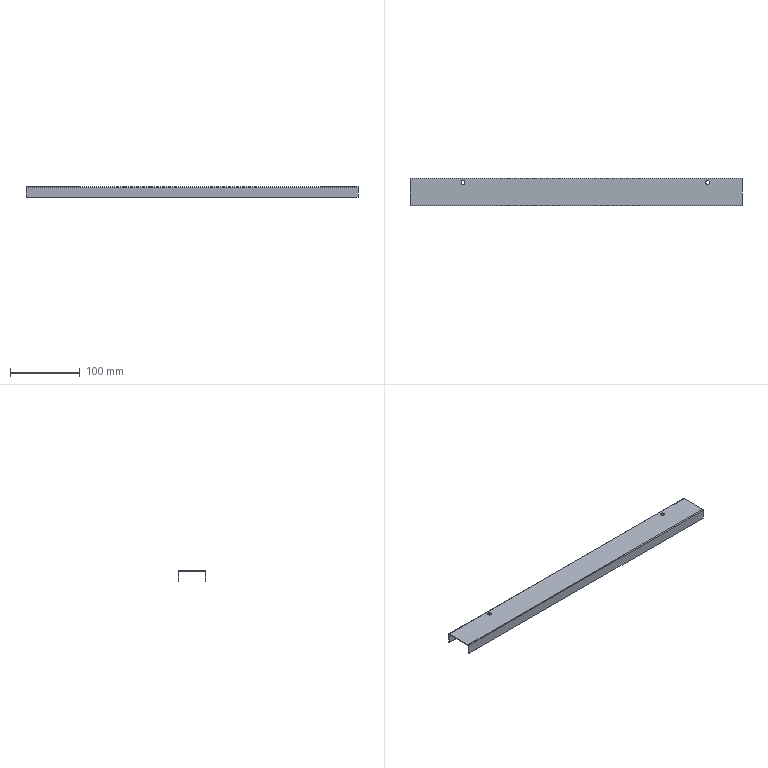Part | SolidWorks | features SplitBody 1 | 1 solid | 26 faces | box 475 x 40 x 15 mm | volume 32008 mm3 | plane 18 | cylinder 8 | commonest cylinder face diameters 5.5 x4 0.2 x2 2.2 x2
STEP:
#1=CARTESIAN_POINT('',(103.5,1393.5,274.));
#2=VERTEX_POINT('',#1);
#3=CARTESIAN_POINT('',(98.,1393.5,274.));
#4=VERTEX_POINT('',#3);
#5=CARTESIAN_POINT('',(100.75,1393.5,274.));
#6=DIRECTION('',(0.,0.,-1.));
#7=DIRECTION('',(-1.,0.,0.));
#8=AXIS2_PLACEMENT_3D('',#5,#6,#7);
#9=CIRCLE('',#8,2.75);
#10=EDGE_CURVE('',#2,#4,#9,.T.);
#11=ORIENTED_EDGE('',*,*,#10,.T.);
#12=CARTESIAN_POINT('',(98.,1393.5,275.));
#13=VERTEX_POINT('',#12);
#14=CARTESIAN_POINT('',(98.,1393.5,265.));
#15=DIRECTION('',(0.,0.,1.));
#16=VECTOR('',#15,1000.);
#17=LINE('',#14,#16);
#18=EDGE_CURVE('',#4,#13,#17,.T.);
#19=ORIENTED_EDGE('',*,*,#18,.T.);
#20=CARTESIAN_POINT('',(103.5,1393.5,275.));
#21=VERTEX_POINT('',#20);
#22=CARTESIAN_POINT('',(100.75,1393.5,275.));
#23=DIRECTION('',(0.,0.,1.));
#24=DIRECTION('',(1.,0.,0.));
#25=AXIS2_PLACEMENT_3D('',#22,#23,#24);
#26=CIRCLE('',#25,2.75);
#27=EDGE_CURVE('',#13,#21,#26,.T.);
#28=ORIENTED_EDGE('',*,*,#27,.T.);
#29=CARTESIAN_POINT('',(103.5,1393.5,265.));
#30=DIRECTION('',(0.,0.,1.));
#31=VECTOR('',#30,1000.);
#32=LINE('',#29,#31);
#33=EDGE_CURVE('',#2,#21,#32,.T.);
#34=ORIENTED_EDGE('',*,*,#33,.F.);
#35=EDGE_LOOP('',(#11,#19,#28,#34));
#36=FACE_OUTER_BOUND('',#35,.T.);
#37=CARTESIAN_POINT('',(100.75,1393.5,265.));
#38=DIRECTION('',(0.,0.,1.));
#39=DIRECTION('',(1.,0.,0.));
#40=AXIS2_PLACEMENT_3D('',#37,#38,#39);
#41=CYLINDRICAL_SURFACE('',#40,2.75);
#42=ADVANCED_FACE('',(#36),#41,.F.);
#43=CARTESIAN_POINT('',(453.5,1393.5,274.));
#44=VERTEX_POINT('',#43);
#45=CARTESIAN_POINT('',(448.,1393.5,274.));
#46=VERTEX_POINT('',#45);
#47=CARTESIAN_POINT('',(450.75,1393.5,274.));
#48=DIRECTION('',(0.,0.,-1.));
#49=DIRECTION('',(-1.,0.,0.));
#50=AXIS2_PLACEMENT_3D('',#47,#48,#49);
#51=CIRCLE('',#50,2.75);
#52=EDGE_CURVE('',#44,#46,#51,.T.);
#53=ORIENTED_EDGE('',*,*,#52,.T.);
#54=CARTESIAN_POINT('',(448.,1393.5,275.));
#55=VERTEX_POINT('',#54);
#56=CARTESIAN_POINT('',(448.,1393.5,265.));
#57=DIRECTION('',(0.,0.,1.));
#58=VECTOR('',#57,1000.);
#59=LINE('',#56,#58);
#60=EDGE_CURVE('',#46,#55,#59,.T.);
#61=ORIENTED_EDGE('',*,*,#60,.T.);
#62=CARTESIAN_POINT('',(453.5,1393.5,275.));
#63=VERTEX_POINT('',#62);
#64=CARTESIAN_POINT('',(450.75,1393.5,275.));
#65=DIRECTION('',(0.,0.,1.));
#66=DIRECTION('',(1.,0.,0.));
#67=AXIS2_PLACEMENT_3D('',#64,#65,#66);
#68=CIRCLE('',#67,2.75);
#69=EDGE_CURVE('',#55,#63,#68,.T.);
#70=ORIENTED_EDGE('',*,*,#69,.T.);
#71=CARTESIAN_POINT('',(453.5,1393.5,265.));
#72=DIRECTION('',(0.,0.,1.));
#73=VECTOR('',#72,1000.);
#74=LINE('',#71,#73);
#75=EDGE_CURVE('',#44,#63,#74,.T.);
#76=ORIENTED_EDGE('',*,*,#75,.F.);
#77=EDGE_LOOP('',(#53,#61,#70,#76));
#78=FACE_OUTER_BOUND('',#77,.T.);
#79=CARTESIAN_POINT('',(450.75,1393.5,265.));
#80=DIRECTION('',(0.,0.,1.));
#81=DIRECTION('',(1.,0.,0.));
#82=AXIS2_PLACEMENT_3D('',#79,#80,#81);
#83=CYLINDRICAL_SURFACE('',#82,2.75);
#84=ADVANCED_FACE('',(#78),#83,.F.);
#85=CARTESIAN_POINT('',(25.,1398.9,275.));
#86=VERTEX_POINT('',#85);
#87=CARTESIAN_POINT('',(25.,1398.9,274.));
#88=VERTEX_POINT('',#87);
#89=CARTESIAN_POINT('',(25.,1398.9,275.));
#90=DIRECTION('',(0.,0.,-1.));
#91=VECTOR('',#90,1000.);
#92=LINE('',#89,#91);
#93=EDGE_CURVE('',#86,#88,#92,.T.);
#94=ORIENTED_EDGE('',*,*,#93,.F.);
#95=CARTESIAN_POINT('',(25.,1400.,273.9));
#96=VERTEX_POINT('',#95);
#97=CARTESIAN_POINT('',(25.,1398.9,273.9));
#98=DIRECTION('',(1.,0.,0.));
#99=DIRECTION('',(0.,0.,1.));
#100=AXIS2_PLACEMENT_3D('',#97,#98,#99);
#101=CIRCLE('',#100,1.1);
#102=EDGE_CURVE('',#96,#86,#101,.T.);
#103=ORIENTED_EDGE('',*,*,#102,.F.);
#104=CARTESIAN_POINT('',(25.,1399.,273.9));
#105=VERTEX_POINT('',#104);
#106=CARTESIAN_POINT('',(25.,1399.,273.9));
#107=DIRECTION('',(0.,1.,0.));
#108=VECTOR('',#107,1000.);
#109=LINE('',#106,#108);
#110=EDGE_CURVE('',#105,#96,#109,.T.);
#111=ORIENTED_EDGE('',*,*,#110,.F.);
#112=CARTESIAN_POINT('',(25.,1398.9,273.9));
#113=DIRECTION('',(1.,0.,0.));
#114=DIRECTION('',(0.,0.,-1.));
#115=AXIS2_PLACEMENT_3D('',#112,#113,#114);
#116=CIRCLE('',#115,0.1);
#117=EDGE_CURVE('',#105,#88,#116,.T.);
#118=ORIENTED_EDGE('',*,*,#117,.T.);
#119=EDGE_LOOP('',(#94,#103,#111,#118));
#120=FACE_OUTER_BOUND('',#119,.T.);
#121=CARTESIAN_POINT('',(25.,1398.9,275.));
#122=DIRECTION('',(-1.,0.,0.));
#123=DIRECTION('',(0.,0.,1.));
#124=AXIS2_PLACEMENT_3D('',#121,#122,#123);
#125=PLANE('',#124);
#126=ADVANCED_FACE('',(#120),#125,.T.);
#127=CARTESIAN_POINT('',(25.,1361.1,275.));
#128=VERTEX_POINT('',#127);
#129=CARTESIAN_POINT('',(25.,1400.,275.));
#130=DIRECTION('',(0.,-1.,0.));
#131=VECTOR('',#130,1000.);
#132=LINE('',#129,#131);
#133=EDGE_CURVE('',#86,#128,#132,.T.);
#134=ORIENTED_EDGE('',*,*,#133,.F.);
#135=ORIENTED_EDGE('',*,*,#93,.T.);
#136=CARTESIAN_POINT('',(25.,1361.1,274.));
#137=VERTEX_POINT('',#136);
#138=CARTESIAN_POINT('',(25.,1400.,274.));
#139=DIRECTION('',(0.,-1.,0.));
#140=VECTOR('',#139,1000.);
#141=LINE('',#138,#140);
#142=EDGE_CURVE('',#88,#137,#141,.T.);
#143=ORIENTED_EDGE('',*,*,#142,.T.);
#144=CARTESIAN_POINT('',(25.,1361.1,274.));
#145=DIRECTION('',(0.,0.,1.));
#146=VECTOR('',#145,1000.);
#147=LINE('',#144,#146);
#148=EDGE_CURVE('',#137,#128,#147,.T.);
#149=ORIENTED_EDGE('',*,*,#148,.T.);
#150=EDGE_LOOP('',(#134,#135,#143,#149));
#151=FACE_OUTER_BOUND('',#150,.T.);
#152=CARTESIAN_POINT('',(25.,1399.,273.9));
#153=DIRECTION('',(-1.,0.,0.));
#154=DIRECTION('',(0.,0.,1.));
#155=AXIS2_PLACEMENT_3D('',#152,#153,#154);
#156=PLANE('',#155);
#157=ADVANCED_FACE('',(#151),#156,.T.);
#158=CARTESIAN_POINT('',(25.,1360.,273.9));
#159=VERTEX_POINT('',#158);
#160=CARTESIAN_POINT('',(25.,1361.,273.9));
#161=VERTEX_POINT('',#160);
#162=CARTESIAN_POINT('',(25.,1360.,273.9));
#163=DIRECTION('',(0.,1.,0.));
#164=VECTOR('',#163,1000.);
#165=LINE('',#162,#164);
#166=EDGE_CURVE('',#159,#161,#165,.T.);
#167=ORIENTED_EDGE('',*,*,#166,.F.);
#168=CARTESIAN_POINT('',(25.,1361.1,273.9));
#169=DIRECTION('',(1.,0.,0.));
#170=DIRECTION('',(0.,0.,1.));
#171=AXIS2_PLACEMENT_3D('',#168,#169,#170);
#172=CIRCLE('',#171,1.1);
#173=EDGE_CURVE('',#128,#159,#172,.T.);
#174=ORIENTED_EDGE('',*,*,#173,.F.);
#175=ORIENTED_EDGE('',*,*,#148,.F.);
#176=CARTESIAN_POINT('',(25.,1361.1,273.9));
#177=DIRECTION('',(1.,0.,0.));
#178=DIRECTION('',(0.,0.,-1.));
#179=AXIS2_PLACEMENT_3D('',#176,#177,#178);
#180=CIRCLE('',#179,0.1);
#181=EDGE_CURVE('',#137,#161,#180,.T.);
#182=ORIENTED_EDGE('',*,*,#181,.T.);
#183=EDGE_LOOP('',(#167,#174,#175,#182));
#184=FACE_OUTER_BOUND('',#183,.T.);
#185=CARTESIAN_POINT('',(25.,1360.,273.9));
#186=DIRECTION('',(-1.,0.,0.));
#187=DIRECTION('',(0.,0.,1.));
#188=AXIS2_PLACEMENT_3D('',#185,#186,#187);
#189=PLANE('',#188);
#190=ADVANCED_FACE('',(#184),#189,.T.);
#191=CARTESIAN_POINT('',(25.,1360.,260.));
#192=VERTEX_POINT('',#191);
#193=CARTESIAN_POINT('',(25.,1360.,275.));
#194=DIRECTION('',(0.,0.,-1.));
#195=VECTOR('',#194,1000.);
#196=LINE('',#193,#195);
#197=EDGE_CURVE('',#159,#192,#196,.T.);
#198=ORIENTED_EDGE('',*,*,#197,.F.);
#199=ORIENTED_EDGE('',*,*,#166,.T.);
#200=CARTESIAN_POINT('',(25.,1361.,260.));
#201=VERTEX_POINT('',#200);
#202=CARTESIAN_POINT('',(25.,1361.,275.));
#203=DIRECTION('',(0.,0.,-1.));
#204=VECTOR('',#203,1000.);
#205=LINE('',#202,#204);
#206=EDGE_CURVE('',#161,#201,#205,.T.);
#207=ORIENTED_EDGE('',*,*,#206,.T.);
#208=CARTESIAN_POINT('',(25.,1361.,260.));
#209=DIRECTION('',(0.,-1.,0.));
#210=VECTOR('',#209,1000.);
#211=LINE('',#208,#210);
#212=EDGE_CURVE('',#201,#192,#211,.T.);
#213=ORIENTED_EDGE('',*,*,#212,.T.);
#214=EDGE_LOOP('',(#198,#199,#207,#213));
#215=FACE_OUTER_BOUND('',#214,.T.);
#216=CARTESIAN_POINT('',(25.,1361.1,274.));
#217=DIRECTION('',(-1.,0.,0.));
#218=DIRECTION('',(0.,0.,1.));
#219=AXIS2_PLACEMENT_3D('',#216,#217,#218);
#220=PLANE('',#219);
#221=ADVANCED_FACE('',(#215),#220,.T.);
#222=CARTESIAN_POINT('',(500.,1360.,273.9));
#223=VERTEX_POINT('',#222);
#224=CARTESIAN_POINT('',(500.,1360.,260.));
#225=VERTEX_POINT('',#224);
#226=CARTESIAN_POINT('',(500.,1360.,275.));
#227=DIRECTION('',(0.,0.,-1.));
#228=VECTOR('',#227,1000.);
#229=LINE('',#226,#228);
#230=EDGE_CURVE('',#223,#225,#229,.T.);
#231=ORIENTED_EDGE('',*,*,#230,.F.);
#232=CARTESIAN_POINT('',(542.72,1360.,273.9));
#233=DIRECTION('',(-1.,0.,0.));
#234=VECTOR('',#233,1000.);
#235=LINE('',#232,#234);
#236=EDGE_CURVE('',#223,#159,#235,.T.);
#237=ORIENTED_EDGE('',*,*,#236,.T.);
#238=ORIENTED_EDGE('',*,*,#197,.T.);
#239=CARTESIAN_POINT('',(542.72,1360.,260.));
#240=DIRECTION('',(-1.,0.,0.));
#241=VECTOR('',#240,1000.);
#242=LINE('',#239,#241);
#243=EDGE_CURVE('',#225,#192,#242,.T.);
#244=ORIENTED_EDGE('',*,*,#243,.F.);
#245=EDGE_LOOP('',(#231,#237,#238,#244));
#246=FACE_OUTER_BOUND('',#245,.T.);
#247=CARTESIAN_POINT('',(542.72,1360.,275.));
#248=DIRECTION('',(0.,1.,0.));
#249=DIRECTION('',(-1.,0.,0.));
#250=AXIS2_PLACEMENT_3D('',#247,#248,#249);
#251=PLANE('',#250);
#252=ADVANCED_FACE('',(#246),#251,.F.);
#253=CARTESIAN_POINT('',(500.,1361.,260.));
#254=VERTEX_POINT('',#253);
#255=CARTESIAN_POINT('',(542.72,1361.,260.));
#256=DIRECTION('',(-1.,0.,0.));
#257=VECTOR('',#256,1000.);
#258=LINE('',#255,#257);
#259=EDGE_CURVE('',#254,#201,#258,.T.);
#260=ORIENTED_EDGE('',*,*,#259,.F.);
#261=CARTESIAN_POINT('',(500.,1361.,260.));
#262=DIRECTION('',(0.,-1.,0.));
#263=VECTOR('',#262,1000.);
#264=LINE('',#261,#263);
#265=EDGE_CURVE('',#254,#225,#264,.T.);
#266=ORIENTED_EDGE('',*,*,#265,.T.);
#267=ORIENTED_EDGE('',*,*,#243,.T.);
#268=ORIENTED_EDGE('',*,*,#212,.F.);
#269=EDGE_LOOP('',(#260,#266,#267,#268));
#270=FACE_OUTER_BOUND('',#269,.T.);
#271=CARTESIAN_POINT('',(542.72,1361.,260.));
#272=DIRECTION('',(0.,0.,-1.));
#273=DIRECTION('',(-1.,0.,0.));
#274=AXIS2_PLACEMENT_3D('',#271,#272,#273);
#275=PLANE('',#274);
#276=ADVANCED_FACE('',(#270),#275,.T.);
#277=CARTESIAN_POINT('',(500.,1361.,273.9));
#278=VERTEX_POINT('',#277);
#279=CARTESIAN_POINT('',(542.72,1361.,273.9));
#280=DIRECTION('',(-1.,0.,0.));
#281=VECTOR('',#280,1000.);
#282=LINE('',#279,#281);
#283=EDGE_CURVE('',#278,#161,#282,.T.);
#284=ORIENTED_EDGE('',*,*,#283,.F.);
#285=CARTESIAN_POINT('',(500.,1361.,275.));
#286=DIRECTION('',(0.,0.,-1.));
#287=VECTOR('',#286,1000.);
#288=LINE('',#285,#287);
#289=EDGE_CURVE('',#278,#254,#288,.T.);
#290=ORIENTED_EDGE('',*,*,#289,.T.);
#291=ORIENTED_EDGE('',*,*,#259,.T.);
#292=ORIENTED_EDGE('',*,*,#206,.F.);
#293=EDGE_LOOP('',(#284,#290,#291,#292));
#294=FACE_OUTER_BOUND('',#293,.T.);
#295=CARTESIAN_POINT('',(542.72,1361.,275.));
#296=DIRECTION('',(0.,1.,0.));
#297=DIRECTION('',(-1.,0.,0.));
#298=AXIS2_PLACEMENT_3D('',#295,#296,#297);
#299=PLANE('',#298);
#300=ADVANCED_FACE('',(#294),#299,.T.);
#301=CARTESIAN_POINT('',(500.,1361.1,274.));
#302=VERTEX_POINT('',#301);
#303=CARTESIAN_POINT('',(542.72,1361.1,274.));
#304=DIRECTION('',(-1.,0.,0.));
#305=VECTOR('',#304,1000.);
#306=LINE('',#303,#305);
#307=EDGE_CURVE('',#302,#137,#306,.T.);
#308=ORIENTED_EDGE('',*,*,#307,.F.);
#309=CARTESIAN_POINT('',(500.,1361.1,273.9));
#310=DIRECTION('',(-1.,0.,0.));
#311=DIRECTION('',(0.,0.,1.));
#312=AXIS2_PLACEMENT_3D('',#309,#310,#311);
#313=CIRCLE('',#312,0.1);
#314=EDGE_CURVE('',#278,#302,#313,.T.);
#315=ORIENTED_EDGE('',*,*,#314,.F.);
#316=ORIENTED_EDGE('',*,*,#283,.T.);
#317=ORIENTED_EDGE('',*,*,#181,.F.);
#318=EDGE_LOOP('',(#308,#315,#316,#317));
#319=FACE_OUTER_BOUND('',#318,.T.);
#320=CARTESIAN_POINT('',(542.72,1361.1,273.9));
#321=DIRECTION('',(-1.,0.,0.));
#322=DIRECTION('',(0.,0.,1.));
#323=AXIS2_PLACEMENT_3D('',#320,#321,#322);
#324=CYLINDRICAL_SURFACE('',#323,0.1);
#325=ADVANCED_FACE('',(#319),#324,.F.);
#326=ORIENTED_EDGE('',*,*,#10,.F.);
#327=CARTESIAN_POINT('',(100.75,1393.5,274.));
#328=DIRECTION('',(0.,0.,-1.));
#329=DIRECTION('',(-1.,0.,0.));
#330=AXIS2_PLACEMENT_3D('',#327,#328,#329);
#331=CIRCLE('',#330,2.75);
#332=EDGE_CURVE('',#4,#2,#331,.T.);
#333=ORIENTED_EDGE('',*,*,#332,.F.);
#334=EDGE_LOOP('',(#326,#333));
#335=FACE_BOUND('',#334,.T.);
#336=ORIENTED_EDGE('',*,*,#52,.F.);
#337=CARTESIAN_POINT('',(450.75,1393.5,274.));
#338=DIRECTION('',(0.,0.,-1.));
#339=DIRECTION('',(-1.,0.,0.));
#340=AXIS2_PLACEMENT_3D('',#337,#338,#339);
#341=CIRCLE('',#340,2.75);
#342=EDGE_CURVE('',#46,#44,#341,.T.);
#343=ORIENTED_EDGE('',*,*,#342,.F.);
#344=EDGE_LOOP('',(#336,#343));
#345=FACE_BOUND('',#344,.T.);
#346=CARTESIAN_POINT('',(500.,1398.9,274.));
#347=VERTEX_POINT('',#346);
#348=CARTESIAN_POINT('',(542.72,1398.9,274.));
#349=DIRECTION('',(-1.,0.,0.));
#350=VECTOR('',#349,1000.);
#351=LINE('',#348,#350);
#352=EDGE_CURVE('',#347,#88,#351,.T.);
#353=ORIENTED_EDGE('',*,*,#352,.F.);
#354=CARTESIAN_POINT('',(500.,1400.,274.));
#355=DIRECTION('',(0.,-1.,0.));
#356=VECTOR('',#355,1000.);
#357=LINE('',#354,#356);
#358=EDGE_CURVE('',#347,#302,#357,.T.);
#359=ORIENTED_EDGE('',*,*,#358,.T.);
#360=ORIENTED_EDGE('',*,*,#307,.T.);
#361=ORIENTED_EDGE('',*,*,#142,.F.);
#362=EDGE_LOOP('',(#353,#359,#360,#361));
#363=FACE_OUTER_BOUND('',#362,.T.);
#364=CARTESIAN_POINT('',(542.72,1400.,274.));
#365=DIRECTION('',(0.,0.,-1.));
#366=DIRECTION('',(-1.,0.,0.));
#367=AXIS2_PLACEMENT_3D('',#364,#365,#366);
#368=PLANE('',#367);
#369=ADVANCED_FACE('',(#335,#345,#363),#368,.T.);
#370=CARTESIAN_POINT('',(500.,1399.,273.9));
#371=VERTEX_POINT('',#370);
#372=CARTESIAN_POINT('',(542.72,1399.,273.9));
#373=DIRECTION('',(-1.,0.,0.));
#374=VECTOR('',#373,1000.);
#375=LINE('',#372,#374);
#376=EDGE_CURVE('',#371,#105,#375,.T.);
#377=ORIENTED_EDGE('',*,*,#376,.F.);
#378=CARTESIAN_POINT('',(500.,1398.9,273.9));
#379=DIRECTION('',(-1.,0.,0.));
#380=DIRECTION('',(0.,0.,1.));
#381=AXIS2_PLACEMENT_3D('',#378,#379,#380);
#382=CIRCLE('',#381,0.1);
#383=EDGE_CURVE('',#347,#371,#382,.T.);
#384=ORIENTED_EDGE('',*,*,#383,.F.);
#385=ORIENTED_EDGE('',*,*,#352,.T.);
#386=ORIENTED_EDGE('',*,*,#117,.F.);
#387=EDGE_LOOP('',(#377,#384,#385,#386));
#388=FACE_OUTER_BOUND('',#387,.T.);
#389=CARTESIAN_POINT('',(542.72,1398.9,273.9));
#390=DIRECTION('',(-1.,0.,0.));
#391=DIRECTION('',(0.,0.,1.));
#392=AXIS2_PLACEMENT_3D('',#389,#390,#391);
#393=CYLINDRICAL_SURFACE('',#392,0.1);
#394=ADVANCED_FACE('',(#388),#393,.F.);
#395=CARTESIAN_POINT('',(500.,1399.,260.));
#396=VERTEX_POINT('',#395);
#397=CARTESIAN_POINT('',(25.,1399.,260.));
#398=VERTEX_POINT('',#397);
#399=CARTESIAN_POINT('',(542.72,1399.,260.));
#400=DIRECTION('',(-1.,0.,0.));
#401=VECTOR('',#400,1000.);
#402=LINE('',#399,#401);
#403=EDGE_CURVE('',#396,#398,#402,.T.);
#404=ORIENTED_EDGE('',*,*,#403,.F.);
#405=CARTESIAN_POINT('',(500.,1399.,260.));
#406=DIRECTION('',(0.,0.,1.));
#407=VECTOR('',#406,1000.);
#408=LINE('',#405,#407);
#409=EDGE_CURVE('',#396,#371,#408,.T.);
#410=ORIENTED_EDGE('',*,*,#409,.T.);
#411=ORIENTED_EDGE('',*,*,#376,.T.);
#412=CARTESIAN_POINT('',(25.,1399.,260.));
#413=DIRECTION('',(0.,0.,1.));
#414=VECTOR('',#413,1000.);
#415=LINE('',#412,#414);
#416=EDGE_CURVE('',#398,#105,#415,.T.);
#417=ORIENTED_EDGE('',*,*,#416,.F.);
#418=EDGE_LOOP('',(#404,#410,#411,#417));
#419=FACE_OUTER_BOUND('',#418,.T.);
#420=CARTESIAN_POINT('',(542.72,1399.,260.));
#421=DIRECTION('',(0.,-1.,0.));
#422=DIRECTION('',(1.,0.,0.));
#423=AXIS2_PLACEMENT_3D('',#420,#421,#422);
#424=PLANE('',#423);
#425=ADVANCED_FACE('',(#419),#424,.T.);
#426=CARTESIAN_POINT('',(500.,1400.,260.));
#427=VERTEX_POINT('',#426);
#428=CARTESIAN_POINT('',(25.,1400.,260.));
#429=VERTEX_POINT('',#428);
#430=CARTESIAN_POINT('',(542.72,1400.,260.));
#431=DIRECTION('',(-1.,0.,0.));
#432=VECTOR('',#431,1000.);
#433=LINE('',#430,#432);
#434=EDGE_CURVE('',#427,#429,#433,.T.);
#435=ORIENTED_EDGE('',*,*,#434,.F.);
#436=CARTESIAN_POINT('',(500.,1400.,260.));
#437=DIRECTION('',(0.,-1.,0.));
#438=VECTOR('',#437,1000.);
#439=LINE('',#436,#438);
#440=EDGE_CURVE('',#427,#396,#439,.T.);
#441=ORIENTED_EDGE('',*,*,#440,.T.);
#442=ORIENTED_EDGE('',*,*,#403,.T.);
#443=CARTESIAN_POINT('',(25.,1400.,260.));
#444=DIRECTION('',(0.,-1.,0.));
#445=VECTOR('',#444,1000.);
#446=LINE('',#443,#445);
#447=EDGE_CURVE('',#429,#398,#446,.T.);
#448=ORIENTED_EDGE('',*,*,#447,.F.);
#449=EDGE_LOOP('',(#435,#441,#442,#448));
#450=FACE_OUTER_BOUND('',#449,.T.);
#451=CARTESIAN_POINT('',(542.72,1400.,260.));
#452=DIRECTION('',(0.,0.,-1.));
#453=DIRECTION('',(-1.,0.,0.));
#454=AXIS2_PLACEMENT_3D('',#451,#452,#453);
#455=PLANE('',#454);
#456=ADVANCED_FACE('',(#450),#455,.T.);
#457=CARTESIAN_POINT('',(500.,1400.,273.9));
#458=VERTEX_POINT('',#457);
#459=CARTESIAN_POINT('',(500.,1400.,260.));
#460=DIRECTION('',(0.,0.,1.));
#461=VECTOR('',#460,1000.);
#462=LINE('',#459,#461);
#463=EDGE_CURVE('',#427,#458,#462,.T.);
#464=ORIENTED_EDGE('',*,*,#463,.F.);
#465=ORIENTED_EDGE('',*,*,#434,.T.);
#466=CARTESIAN_POINT('',(25.,1400.,260.));
#467=DIRECTION('',(0.,0.,1.));
#468=VECTOR('',#467,1000.);
#469=LINE('',#466,#468);
#470=EDGE_CURVE('',#429,#96,#469,.T.);
#471=ORIENTED_EDGE('',*,*,#470,.T.);
#472=CARTESIAN_POINT('',(542.72,1400.,273.9));
#473=DIRECTION('',(-1.,0.,0.));
#474=VECTOR('',#473,1000.);
#475=LINE('',#472,#474);
#476=EDGE_CURVE('',#458,#96,#475,.T.);
#477=ORIENTED_EDGE('',*,*,#476,.F.);
#478=EDGE_LOOP('',(#464,#465,#471,#477));
#479=FACE_OUTER_BOUND('',#478,.T.);
#480=CARTESIAN_POINT('',(542.72,1400.,260.));
#481=DIRECTION('',(0.,-1.,0.));
#482=DIRECTION('',(1.,0.,0.));
#483=AXIS2_PLACEMENT_3D('',#480,#481,#482);
#484=PLANE('',#483);
#485=ADVANCED_FACE('',(#479),#484,.F.);
#486=CARTESIAN_POINT('',(500.,1398.9,275.));
#487=VERTEX_POINT('',#486);
#488=CARTESIAN_POINT('',(500.,1398.9,273.9));
#489=DIRECTION('',(1.,0.,0.));
#490=DIRECTION('',(0.,0.,-1.));
#491=AXIS2_PLACEMENT_3D('',#488,#489,#490);
#492=CIRCLE('',#491,1.1);
#493=EDGE_CURVE('',#458,#487,#492,.T.);
#494=ORIENTED_EDGE('',*,*,#493,.F.);
#495=ORIENTED_EDGE('',*,*,#476,.T.);
#496=ORIENTED_EDGE('',*,*,#102,.T.);
#497=CARTESIAN_POINT('',(542.72,1398.9,275.));
#498=DIRECTION('',(-1.,0.,0.));
#499=VECTOR('',#498,1000.);
#500=LINE('',#497,#499);
#501=EDGE_CURVE('',#487,#86,#500,.T.);
#502=ORIENTED_EDGE('',*,*,#501,.F.);
#503=EDGE_LOOP('',(#494,#495,#496,#502));
#504=FACE_OUTER_BOUND('',#503,.T.);
#505=CARTESIAN_POINT('',(542.72,1398.9,273.9));
#506=DIRECTION('',(-1.,0.,0.));
#507=DIRECTION('',(0.,0.,1.));
#508=AXIS2_PLACEMENT_3D('',#505,#506,#507);
#509=CYLINDRICAL_SURFACE('',#508,1.1);
#510=ADVANCED_FACE('',(#504),#509,.T.);
#511=CARTESIAN_POINT('',(100.75,1393.5,275.));
#512=DIRECTION('',(0.,0.,1.));
#513=DIRECTION('',(1.,0.,0.));
#514=AXIS2_PLACEMENT_3D('',#511,#512,#513);
#515=CIRCLE('',#514,2.75);
#516=EDGE_CURVE('',#21,#13,#515,.T.);
#517=ORIENTED_EDGE('',*,*,#516,.F.);
#518=ORIENTED_EDGE('',*,*,#27,.F.);
#519=EDGE_LOOP('',(#517,#518));
#520=FACE_BOUND('',#519,.T.);
#521=CARTESIAN_POINT('',(450.75,1393.5,275.));
#522=DIRECTION('',(0.,0.,1.));
#523=DIRECTION('',(1.,0.,0.));
#524=AXIS2_PLACEMENT_3D('',#521,#522,#523);
#525=CIRCLE('',#524,2.75);
#526=EDGE_CURVE('',#63,#55,#525,.T.);
#527=ORIENTED_EDGE('',*,*,#526,.F.);
#528=ORIENTED_EDGE('',*,*,#69,.F.);
#529=EDGE_LOOP('',(#527,#528));
#530=FACE_BOUND('',#529,.T.);
#531=CARTESIAN_POINT('',(500.,1361.1,275.));
#532=VERTEX_POINT('',#531);
#533=CARTESIAN_POINT('',(500.,1400.,275.));
#534=DIRECTION('',(0.,-1.,0.));
#535=VECTOR('',#534,1000.);
#536=LINE('',#533,#535);
#537=EDGE_CURVE('',#487,#532,#536,.T.);
#538=ORIENTED_EDGE('',*,*,#537,.F.);
#539=ORIENTED_EDGE('',*,*,#501,.T.);
#540=ORIENTED_EDGE('',*,*,#133,.T.);
#541=CARTESIAN_POINT('',(542.72,1361.1,275.));
#542=DIRECTION('',(-1.,0.,0.));
#543=VECTOR('',#542,1000.);
#544=LINE('',#541,#543);
#545=EDGE_CURVE('',#532,#128,#544,.T.);
#546=ORIENTED_EDGE('',*,*,#545,.F.);
#547=EDGE_LOOP('',(#538,#539,#540,#546));
#548=FACE_OUTER_BOUND('',#547,.T.);
#549=CARTESIAN_POINT('',(542.72,1400.,275.));
#550=DIRECTION('',(0.,0.,-1.));
#551=DIRECTION('',(-1.,0.,0.));
#552=AXIS2_PLACEMENT_3D('',#549,#550,#551);
#553=PLANE('',#552);
#554=ADVANCED_FACE('',(#520,#530,#548),#553,.F.);
#555=CARTESIAN_POINT('',(500.,1361.1,273.9));
#556=DIRECTION('',(1.,0.,0.));
#557=DIRECTION('',(0.,0.,-1.));
#558=AXIS2_PLACEMENT_3D('',#555,#556,#557);
#559=CIRCLE('',#558,1.1);
#560=EDGE_CURVE('',#532,#223,#559,.T.);
#561=ORIENTED_EDGE('',*,*,#560,.F.);
#562=ORIENTED_EDGE('',*,*,#545,.T.);
#563=ORIENTED_EDGE('',*,*,#173,.T.);
#564=ORIENTED_EDGE('',*,*,#236,.F.);
#565=EDGE_LOOP('',(#561,#562,#563,#564));
#566=FACE_OUTER_BOUND('',#565,.T.);
#567=CARTESIAN_POINT('',(542.72,1361.1,273.9));
#568=DIRECTION('',(-1.,0.,0.));
#569=DIRECTION('',(0.,0.,1.));
#570=AXIS2_PLACEMENT_3D('',#567,#568,#569);
#571=CYLINDRICAL_SURFACE('',#570,1.1);
#572=ADVANCED_FACE('',(#566),#571,.T.);
#573=ORIENTED_EDGE('',*,*,#416,.T.);
#574=ORIENTED_EDGE('',*,*,#110,.T.);
#575=ORIENTED_EDGE('',*,*,#470,.F.);
#576=ORIENTED_EDGE('',*,*,#447,.T.);
#577=EDGE_LOOP('',(#573,#574,#575,#576));
#578=FACE_OUTER_BOUND('',#577,.T.);
#579=CARTESIAN_POINT('',(25.,1361.1,273.9));
#580=DIRECTION('',(1.,0.,0.));
#581=DIRECTION('',(0.,0.,-1.));
#582=AXIS2_PLACEMENT_3D('',#579,#580,#581);
#583=PLANE('',#582);
#584=ADVANCED_FACE('',(#578),#583,.F.);
#585=ORIENTED_EDGE('',*,*,#537,.T.);
#586=CARTESIAN_POINT('',(500.,1361.1,275.));
#587=DIRECTION('',(0.,0.,-1.));
#588=VECTOR('',#587,1000.);
#589=LINE('',#586,#588);
#590=EDGE_CURVE('',#532,#302,#589,.T.);
#591=ORIENTED_EDGE('',*,*,#590,.T.);
#592=ORIENTED_EDGE('',*,*,#358,.F.);
#593=CARTESIAN_POINT('',(500.,1398.9,275.));
#594=DIRECTION('',(0.,0.,-1.));
#595=VECTOR('',#594,1000.);
#596=LINE('',#593,#595);
#597=EDGE_CURVE('',#487,#347,#596,.T.);
#598=ORIENTED_EDGE('',*,*,#597,.F.);
#599=EDGE_LOOP('',(#585,#591,#592,#598));
#600=FACE_OUTER_BOUND('',#599,.T.);
#601=CARTESIAN_POINT('',(500.,1400.,275.));
#602=DIRECTION('',(1.,0.,0.));
#603=DIRECTION('',(0.,-1.,0.));
#604=AXIS2_PLACEMENT_3D('',#601,#602,#603);
#605=PLANE('',#604);
#606=ADVANCED_FACE('',(#600),#605,.T.);
#607=ORIENTED_EDGE('',*,*,#463,.T.);
#608=CARTESIAN_POINT('',(500.,1400.,273.9));
#609=DIRECTION('',(0.,-1.,0.));
#610=VECTOR('',#609,1000.);
#611=LINE('',#608,#610);
#612=EDGE_CURVE('',#458,#371,#611,.T.);
#613=ORIENTED_EDGE('',*,*,#612,.T.);
#614=ORIENTED_EDGE('',*,*,#409,.F.);
#615=ORIENTED_EDGE('',*,*,#440,.F.);
#616=EDGE_LOOP('',(#607,#613,#614,#615));
#617=FACE_OUTER_BOUND('',#616,.T.);
#618=CARTESIAN_POINT('',(500.,1400.,260.));
#619=DIRECTION('',(1.,0.,0.));
#620=DIRECTION('',(0.,0.,1.));
#621=AXIS2_PLACEMENT_3D('',#618,#619,#620);
#622=PLANE('',#621);
#623=ADVANCED_FACE('',(#617),#622,.T.);
#624=ORIENTED_EDGE('',*,*,#383,.T.);
#625=ORIENTED_EDGE('',*,*,#612,.F.);
#626=ORIENTED_EDGE('',*,*,#493,.T.);
#627=ORIENTED_EDGE('',*,*,#597,.T.);
#628=EDGE_LOOP('',(#624,#625,#626,#627));
#629=FACE_OUTER_BOUND('',#628,.T.);
#630=CARTESIAN_POINT('',(500.,1398.9,273.9));
#631=DIRECTION('',(-1.,0.,0.));
#632=DIRECTION('',(0.,0.,1.));
#633=AXIS2_PLACEMENT_3D('',#630,#631,#632);
#634=PLANE('',#633);
#635=ADVANCED_FACE('',(#629),#634,.F.);
#636=ORIENTED_EDGE('',*,*,#265,.F.);
#637=ORIENTED_EDGE('',*,*,#289,.F.);
#638=CARTESIAN_POINT('',(500.,1361.,273.9));
#639=DIRECTION('',(0.,-1.,0.));
#640=VECTOR('',#639,1000.);
#641=LINE('',#638,#640);
#642=EDGE_CURVE('',#278,#223,#641,.T.);
#643=ORIENTED_EDGE('',*,*,#642,.T.);
#644=ORIENTED_EDGE('',*,*,#230,.T.);
#645=EDGE_LOOP('',(#636,#637,#643,#644));
#646=FACE_OUTER_BOUND('',#645,.T.);
#647=CARTESIAN_POINT('',(500.,1361.,275.));
#648=DIRECTION('',(1.,0.,0.));
#649=DIRECTION('',(0.,0.,-1.));
#650=AXIS2_PLACEMENT_3D('',#647,#648,#649);
#651=PLANE('',#650);
#652=ADVANCED_FACE('',(#646),#651,.T.);
#653=ORIENTED_EDGE('',*,*,#314,.T.);
#654=ORIENTED_EDGE('',*,*,#590,.F.);
#655=ORIENTED_EDGE('',*,*,#560,.T.);
#656=ORIENTED_EDGE('',*,*,#642,.F.);
#657=EDGE_LOOP('',(#653,#654,#655,#656));
#658=FACE_OUTER_BOUND('',#657,.T.);
#659=CARTESIAN_POINT('',(500.,1361.1,273.9));
#660=DIRECTION('',(-1.,0.,0.));
#661=DIRECTION('',(0.,0.,1.));
#662=AXIS2_PLACEMENT_3D('',#659,#660,#661);
#663=PLANE('',#662);
#664=ADVANCED_FACE('',(#658),#663,.F.);
#665=ORIENTED_EDGE('',*,*,#60,.F.);
#666=ORIENTED_EDGE('',*,*,#342,.T.);
#667=ORIENTED_EDGE('',*,*,#75,.T.);
#668=ORIENTED_EDGE('',*,*,#526,.T.);
#669=EDGE_LOOP('',(#665,#666,#667,#668));
#670=FACE_OUTER_BOUND('',#669,.T.);
#671=CARTESIAN_POINT('',(450.75,1393.5,265.));
#672=DIRECTION('',(0.,0.,1.));
#673=DIRECTION('',(1.,0.,0.));
#674=AXIS2_PLACEMENT_3D('',#671,#672,#673);
#675=CYLINDRICAL_SURFACE('',#674,2.75);
#676=ADVANCED_FACE('',(#670),#675,.F.);
#677=ORIENTED_EDGE('',*,*,#18,.F.);
#678=ORIENTED_EDGE('',*,*,#332,.T.);
#679=ORIENTED_EDGE('',*,*,#33,.T.);
#680=ORIENTED_EDGE('',*,*,#516,.T.);
#681=EDGE_LOOP('',(#677,#678,#679,#680));
#682=FACE_OUTER_BOUND('',#681,.T.);
#683=CARTESIAN_POINT('',(100.75,1393.5,265.));
#684=DIRECTION('',(0.,0.,1.));
#685=DIRECTION('',(1.,0.,0.));
#686=AXIS2_PLACEMENT_3D('',#683,#684,#685);
#687=CYLINDRICAL_SURFACE('',#686,2.75);
#688=ADVANCED_FACE('',(#682),#687,.F.);
#689=CLOSED_SHELL('',(#42,#84,#126,#157,#190,#221,#252,#276,#300,#325,#369,#394,#425,#456,#485,#510,#554,#572,#584,#606,#623,#635,#652,#664,#676,#688));
#690=MANIFOLD_SOLID_BREP('',#689);
#691=CARTESIAN_POINT('',(0.,0.,0.));
#692=DIRECTION('',(0.,0.,1.));
#693=DIRECTION('',(1.,0.,0.));
#694=AXIS2_PLACEMENT_3D('',#691,#692,#693);
#695=(LENGTH_UNIT()NAMED_UNIT(*)SI_UNIT(.MILLI.,.METRE.));
#696=UNCERTAINTY_MEASURE_WITH_UNIT(LENGTH_MEASURE(0.00001),#695,'','');
#697=(NAMED_UNIT(*)PLANE_ANGLE_UNIT()SI_UNIT($,.RADIAN.));
#698=(NAMED_UNIT(*)SI_UNIT($,.STERADIAN.)SOLID_ANGLE_UNIT());
#699=(GEOMETRIC_REPRESENTATION_CONTEXT(3)GLOBAL_UNCERTAINTY_ASSIGNED_CONTEXT((#696))GLOBAL_UNIT_ASSIGNED_CONTEXT((#695,#697,#698))REPRESENTATION_CONTEXT('',''));
#700=ADVANCED_BREP_SHAPE_REPRESENTATION('',(#690,#694),#699);